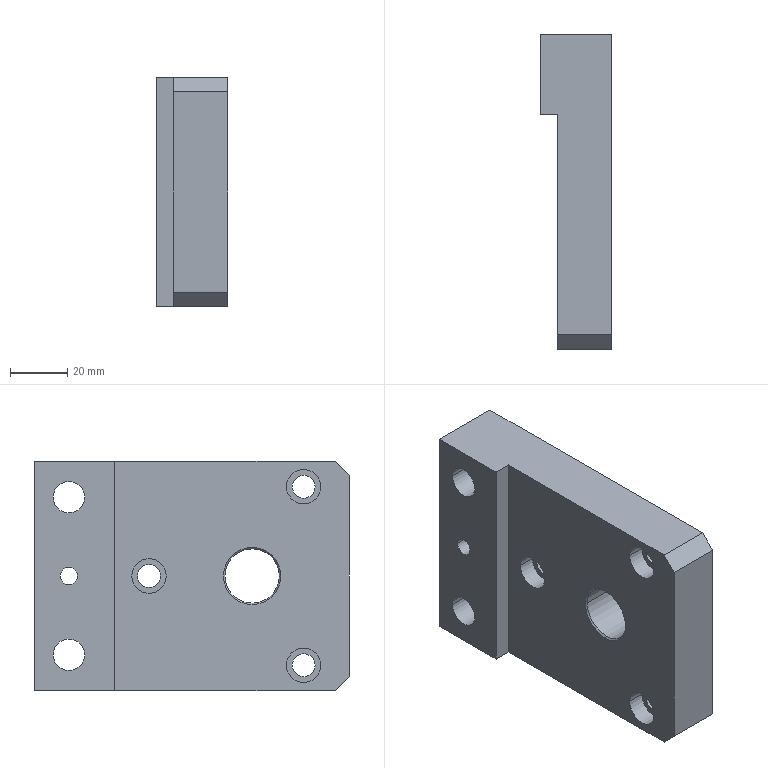Part | STEP file | Cuon T phu H01_10 | 1 solid | 43 faces | box 25 x 110 x 80 mm | volume 162511 mm3 | cylinder 24 | plane 15 | cone 4 | commonest cylinder face diameters 8 x6 12 x6 11 x4 17 x4 6 x2 19 x2